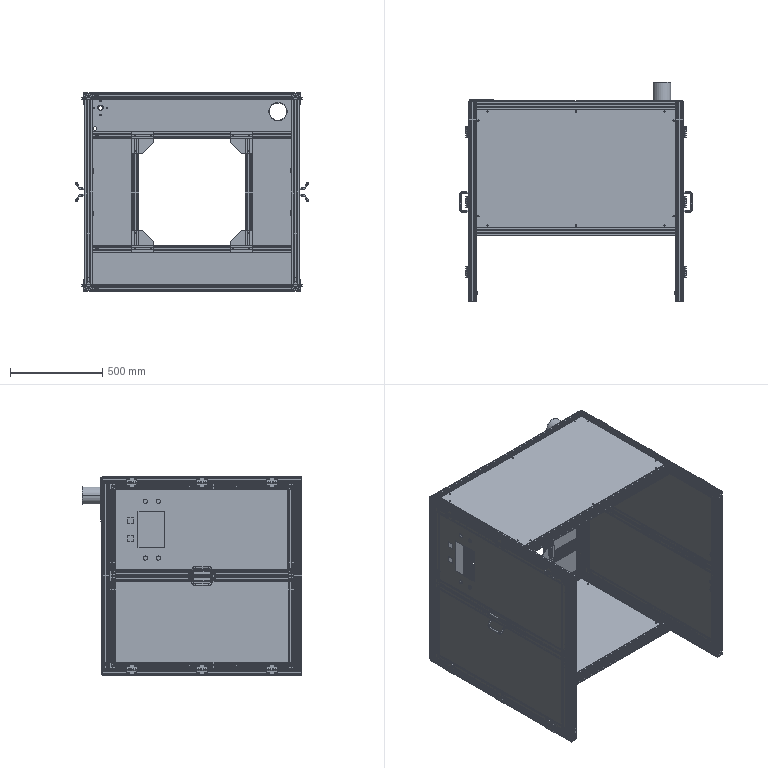Part | SolidWorks | 146 solids | 5151 faces | volume 38823835 mm3 | plane 3186 | cylinder 1766 | cone 163 | torus 24 | spline 8 | sphere 4 | commonest cylinder face diameters 5 x372 7 x294 11 x224 6 x144 6.6 x104 14.5 x72